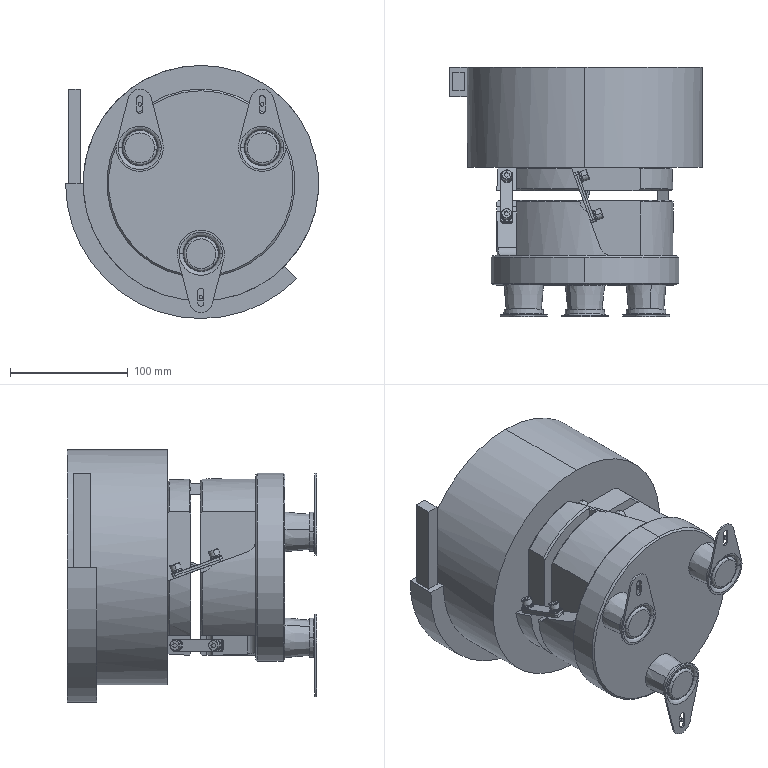Part | SolidWorks | 47 solids | 668 faces | box 215 x 212 x 215 mm | volume 2165561 mm3 | plane 254 | cylinder 233 | torus 108 | cone 73 | commonest cylinder face diameters 4 x32 6 x32 5 x16 5.4 x16 5.5 x16 8.5 x16